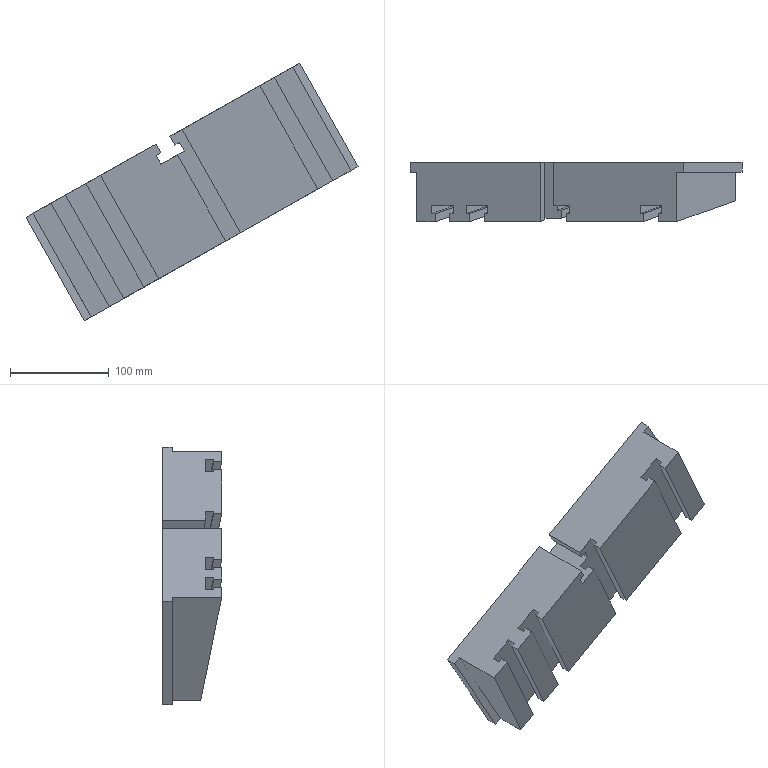Part | STEP file | solid 151 | 1 solid | 50 faces | box 335.969 x 60 x 260.545 mm | volume 1623800 mm3 | plane 47 | spline 3